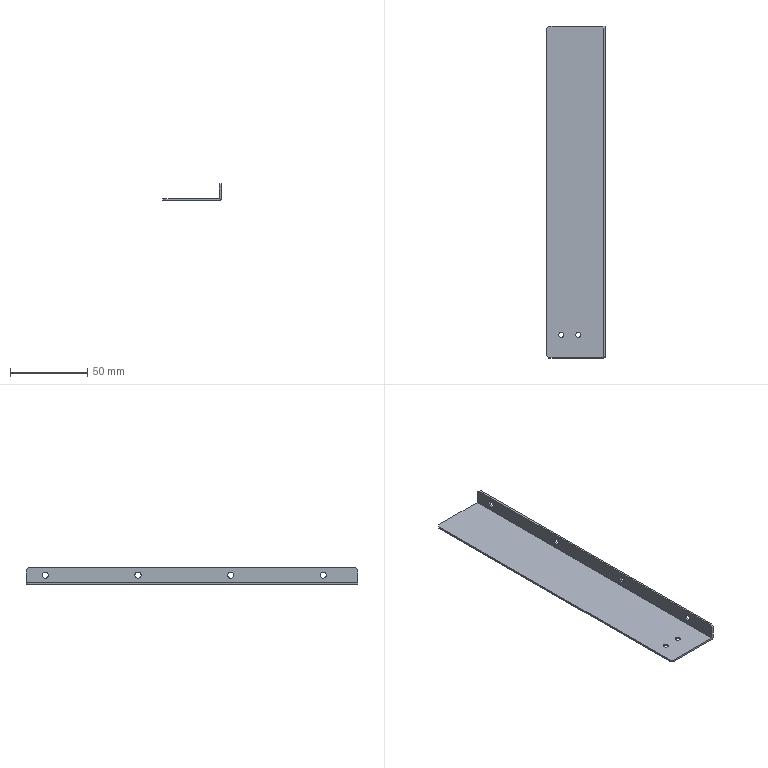Part | STEP file | drag chain support plate | 1 solid | 30 faces | box 38 x 215 x 11 mm | volume 12174 mm3 | plane 16 | cylinder 14 | commonest cylinder face diameters 4 x8 3.3 x4 0.1 x1 2.5 x1